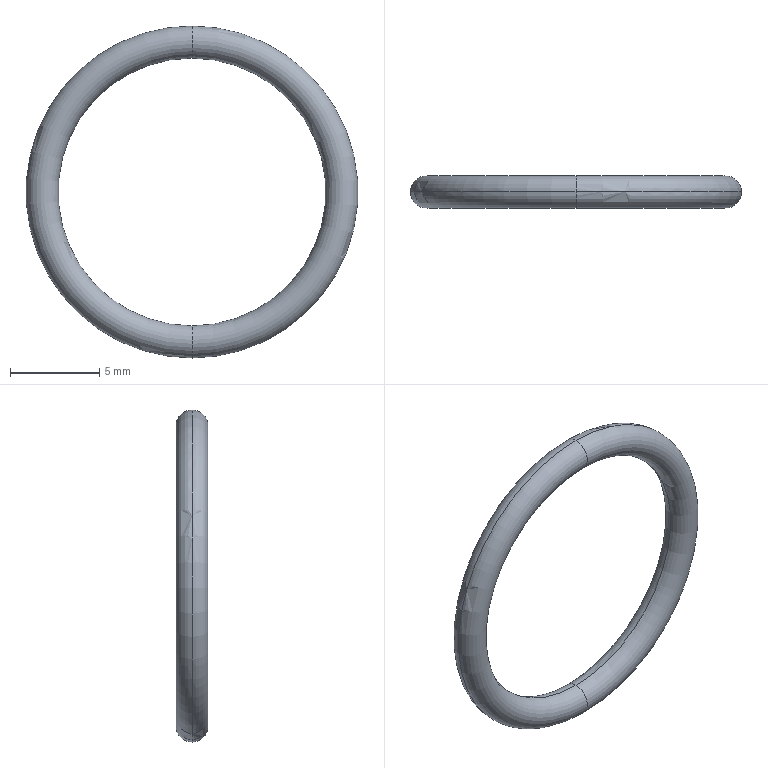Part | STEP file | 1 solid | 4 faces | box 18.6 x 1.8 x 18.6 mm | volume 134.306 mm3 | torus 4
STEP:
#1=CARTESIAN_POINT('',(0.,0.,9.3));
#2=VERTEX_POINT('',#1);
#3=CARTESIAN_POINT('',(0.,0.,7.5));
#4=VERTEX_POINT('',#3);
#5=CARTESIAN_POINT('',(0.,0.,8.4));
#6=DIRECTION('',(1.,0.,0.));
#7=DIRECTION('',(0.,0.,-1.));
#8=AXIS2_PLACEMENT_3D('',#5,#6,#7);
#9=CIRCLE('',#8,0.9);
#10=EDGE_CURVE('',#2,#4,#9,.T.);
#11=ORIENTED_EDGE('',*,*,#10,.F.);
#12=CARTESIAN_POINT('',(0.,0.,-9.3));
#13=VERTEX_POINT('',#12);
#14=CARTESIAN_POINT('',(0.,0.,0.));
#15=DIRECTION('',(0.,-1.,0.));
#16=DIRECTION('',(0.,0.,-1.));
#17=AXIS2_PLACEMENT_3D('',#14,#15,#16);
#18=CIRCLE('',#17,9.3);
#19=EDGE_CURVE('',#2,#13,#18,.T.);
#20=ORIENTED_EDGE('',*,*,#19,.T.);
#21=CARTESIAN_POINT('',(0.,0.,-7.5));
#22=VERTEX_POINT('',#21);
#23=CARTESIAN_POINT('',(0.,0.,-8.4));
#24=DIRECTION('',(-1.,0.,0.));
#25=DIRECTION('',(0.,0.,1.));
#26=AXIS2_PLACEMENT_3D('',#23,#24,#25);
#27=CIRCLE('',#26,0.9);
#28=EDGE_CURVE('',#13,#22,#27,.T.);
#29=ORIENTED_EDGE('',*,*,#28,.T.);
#30=CARTESIAN_POINT('',(0.,0.,0.));
#31=DIRECTION('',(0.,-1.,0.));
#32=DIRECTION('',(0.,0.,-1.));
#33=AXIS2_PLACEMENT_3D('',#30,#31,#32);
#34=CIRCLE('',#33,7.5);
#35=EDGE_CURVE('',#4,#22,#34,.T.);
#36=ORIENTED_EDGE('',*,*,#35,.F.);
#37=EDGE_LOOP('',(#11,#20,#29,#36));
#38=FACE_OUTER_BOUND('',#37,.T.);
#39=CARTESIAN_POINT('',(0.,0.,0.));
#40=DIRECTION('',(0.,-1.,0.));
#41=DIRECTION('',(0.,0.,-1.));
#42=AXIS2_PLACEMENT_3D('',#39,#40,#41);
#43=TOROIDAL_SURFACE('',#42,8.4,0.9);
#44=ADVANCED_FACE('',(#38),#43,.T.);
#45=ORIENTED_EDGE('',*,*,#28,.F.);
#46=CARTESIAN_POINT('',(0.,0.,0.));
#47=DIRECTION('',(0.,-1.,0.));
#48=DIRECTION('',(0.,0.,-1.));
#49=AXIS2_PLACEMENT_3D('',#46,#47,#48);
#50=CIRCLE('',#49,9.3);
#51=EDGE_CURVE('',#13,#2,#50,.T.);
#52=ORIENTED_EDGE('',*,*,#51,.T.);
#53=ORIENTED_EDGE('',*,*,#10,.T.);
#54=CARTESIAN_POINT('',(0.,0.,0.));
#55=DIRECTION('',(0.,-1.,0.));
#56=DIRECTION('',(0.,0.,-1.));
#57=AXIS2_PLACEMENT_3D('',#54,#55,#56);
#58=CIRCLE('',#57,7.5);
#59=EDGE_CURVE('',#22,#4,#58,.T.);
#60=ORIENTED_EDGE('',*,*,#59,.F.);
#61=EDGE_LOOP('',(#45,#52,#53,#60));
#62=FACE_OUTER_BOUND('',#61,.T.);
#63=CARTESIAN_POINT('',(0.,0.,0.));
#64=DIRECTION('',(0.,-1.,0.));
#65=DIRECTION('',(0.,0.,-1.));
#66=AXIS2_PLACEMENT_3D('',#63,#64,#65);
#67=TOROIDAL_SURFACE('',#66,8.4,0.9);
#68=ADVANCED_FACE('',(#62),#67,.T.);
#69=ORIENTED_EDGE('',*,*,#51,.F.);
#70=CARTESIAN_POINT('',(0.,0.,-8.4));
#71=DIRECTION('',(-1.,0.,0.));
#72=DIRECTION('',(0.,0.,1.));
#73=AXIS2_PLACEMENT_3D('',#70,#71,#72);
#74=CIRCLE('',#73,0.9);
#75=EDGE_CURVE('',#22,#13,#74,.T.);
#76=ORIENTED_EDGE('',*,*,#75,.F.);
#77=ORIENTED_EDGE('',*,*,#59,.T.);
#78=CARTESIAN_POINT('',(0.,0.,8.4));
#79=DIRECTION('',(1.,0.,0.));
#80=DIRECTION('',(0.,0.,-1.));
#81=AXIS2_PLACEMENT_3D('',#78,#79,#80);
#82=CIRCLE('',#81,0.9);
#83=EDGE_CURVE('',#4,#2,#82,.T.);
#84=ORIENTED_EDGE('',*,*,#83,.T.);
#85=EDGE_LOOP('',(#69,#76,#77,#84));
#86=FACE_OUTER_BOUND('',#85,.T.);
#87=CARTESIAN_POINT('',(0.,0.,0.));
#88=DIRECTION('',(0.,-1.,0.));
#89=DIRECTION('',(0.,0.,-1.));
#90=AXIS2_PLACEMENT_3D('',#87,#88,#89);
#91=TOROIDAL_SURFACE('',#90,8.4,0.9);
#92=ADVANCED_FACE('',(#86),#91,.T.);
#93=ORIENTED_EDGE('',*,*,#19,.F.);
#94=ORIENTED_EDGE('',*,*,#83,.F.);
#95=ORIENTED_EDGE('',*,*,#35,.T.);
#96=ORIENTED_EDGE('',*,*,#75,.T.);
#97=EDGE_LOOP('',(#93,#94,#95,#96));
#98=FACE_OUTER_BOUND('',#97,.T.);
#99=CARTESIAN_POINT('',(0.,0.,0.));
#100=DIRECTION('',(0.,-1.,0.));
#101=DIRECTION('',(0.,0.,-1.));
#102=AXIS2_PLACEMENT_3D('',#99,#100,#101);
#103=TOROIDAL_SURFACE('',#102,8.4,0.9);
#104=ADVANCED_FACE('',(#98),#103,.T.);
#105=CLOSED_SHELL('',(#44,#68,#92,#104));
#106=MANIFOLD_SOLID_BREP('',#105);
#107=CARTESIAN_POINT('',(0.,0.,0.));
#108=DIRECTION('',(0.,0.,1.));
#109=DIRECTION('',(1.,0.,0.));
#110=AXIS2_PLACEMENT_3D('',#107,#108,#109);
#111=(LENGTH_UNIT()NAMED_UNIT(*)SI_UNIT(.MILLI.,.METRE.));
#112=UNCERTAINTY_MEASURE_WITH_UNIT(LENGTH_MEASURE(0.00001),#111,'','');
#113=(NAMED_UNIT(*)PLANE_ANGLE_UNIT()SI_UNIT($,.RADIAN.));
#114=(NAMED_UNIT(*)SI_UNIT($,.STERADIAN.)SOLID_ANGLE_UNIT());
#115=(GEOMETRIC_REPRESENTATION_CONTEXT(3)GLOBAL_UNCERTAINTY_ASSIGNED_CONTEXT((#112))GLOBAL_UNIT_ASSIGNED_CONTEXT((#111,#113,#114))REPRESENTATION_CONTEXT('',''));
#116=ADVANCED_BREP_SHAPE_REPRESENTATION('',(#106,#110),#115);